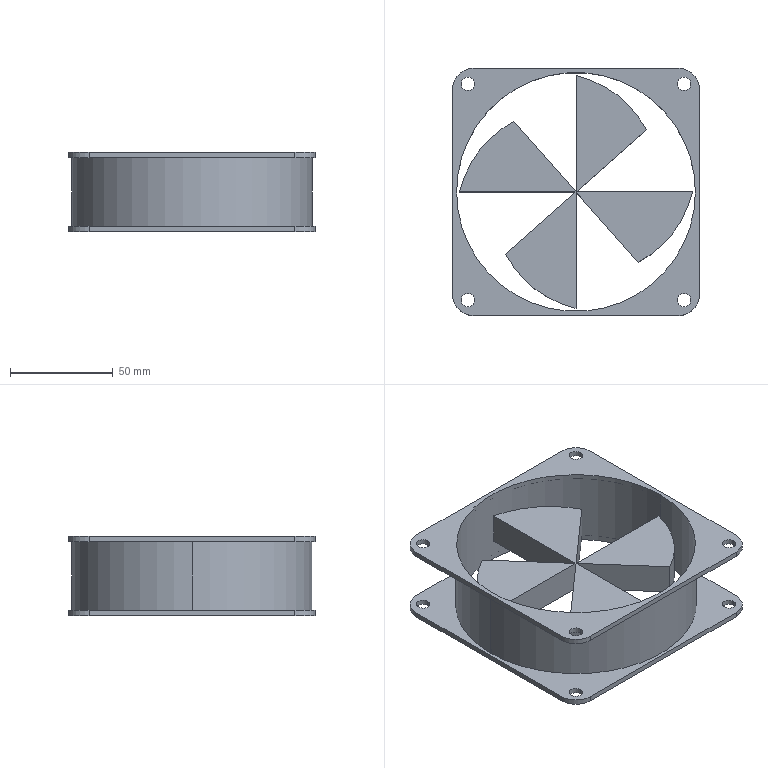Part | SolidWorks | features ICE 3, CirPattern 1, Extrusion 1, Fillet 1, HoleWzd 1, MirrorPattern 1 | 5 solids | 60 faces | box 120 x 120 x 38.5 mm | volume 90385 mm3 | cylinder 32 | plane 28 | commonest cylinder face diameters 6.6 x16 20 x8 103.649 x4 116 x2 117 x2